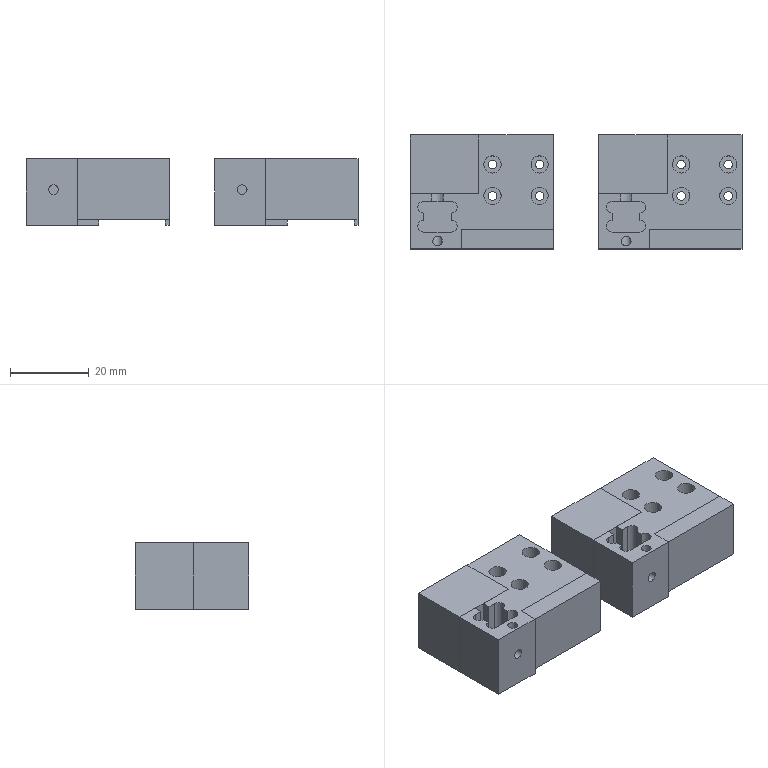NC program | NX | posted with a generic post | part box 84.5 x 29 x 17 mm
Lines 1071 to 2305 of 5162:
(FLOOR_WALL_1 , TOOL : D3)
N2122 T03 M6
N2124 G54
N2126 G17 G0 G90 X-35.75 Y-5.834 B0. C0. S9500 M3
N2128 G43 Z30. H3
N2130 Z1.
N2132 G94 G1 Y-7.2 Z0.928 F1250.
N2134 X-34.75 Z0.876
N2136 Y-5.4 Z0.782
N2138 X-35.75 Z0.729
N2140 Y-7.2 Z0.635
N2142 X-34.75 Z0.583
N2144 Y-5.4 Z0.488
N2146 X-35.75 Z0.436
N2148 Y-7.2 Z0.341
N2150 X-34.75 Z0.289
N2152 Y-5.4 Z0.195
N2154 X-35.75 Z0.142
N2156 Y-7.2 Z0.048
N2158 X-34.75 Z-0.004
N2160 Y-5.4 Z-0.099
N2162 X-35.75 Z-0.151
N2164 Y-6.3 Z-0.198
N2166 Y-7.2
N2168 X-34.75
N2170 Y-5.4
N2172 X-35.75
N2174 Y-6.3
N2176 X-37.25
N2178 Y-7.2
N2180 G2 X-38.75 Y-8.7 R1.5
N2182 G1 X-31.75
N2184 G2 X-33.25 Y-7.2 R1.5
N2186 G1 Y-5.4
N2188 G2 X-31.75 Y-3.9 R1.5
N2190 G1 X-38.75
N2192 G2 X-37.25 Y-5.4 R1.5
N2194 G1 Y-6.3
N2196 Z0.802
N2198 G0 X-35.75 Y-5.834
N2200 G1 Y-7.2 Z0.73
N2202 X-34.75 Z0.678
N2204 Y-5.4 Z0.583
N2206 X-35.75 Z0.531
N2208 Y-7.2 Z0.437
N2210 X-34.75 Z0.384
N2212 Y-5.4 Z0.29
N2214 X-35.75 Z0.237
N2216 Y-7.2 Z0.143
N2218 X-34.75 Z0.091
N2220 Y-5.4 Z-0.004
N2222 X-35.75 Z-0.056
N2224 Y-7.2 Z-0.15
N2226 X-34.75 Z-0.203
N2228 Y-5.4 Z-0.297
N2230 X-35.75 Z-0.35
N2232 Y-6.3 Z-0.397
N2234 Y-7.2
N2236 X-34.75
N2238 Y-5.4
N2240 X-35.75
N2242 Y-6.3
N2244 X-37.25
N2246 Y-7.2
N2248 G2 X-38.75 Y-8.7 R1.5
N2250 G1 X-31.75
N2252 G2 X-33.25 Y-7.2 R1.5
N2254 G1 Y-5.4
N2256 G2 X-31.75 Y-3.9 R1.5
N2258 G1 X-38.75
N2260 G2 X-37.25 Y-5.4 R1.5
N2262 G1 Y-6.3
N2264 Z0.603
N2266 G0 X-35.75 Y-5.834
N2268 G1 Y-7.2 Z0.532
N2270 X-34.75 Z0.479
N2272 Y-5.4 Z0.385
N2274 X-35.75 Z0.333
N2276 Y-7.2 Z0.238
N2278 X-34.75 Z0.186
N2280 Y-5.4 Z0.092
N2282 X-35.75 Z0.039
N2284 Y-7.2 Z-0.055
N2286 X-34.75 Z-0.108
N2288 Y-5.4 Z-0.202
N2290 X-35.75 Z-0.254
N2292 Y-7.2 Z-0.349
N2294 X-34.75 Z-0.401
N2296 Y-5.4 Z-0.495
N2298 X-35.75 Z-0.548
N2300 Y-6.3 Z-0.595
N2302 Y-7.2
N2304 X-34.75
N2306 Y-5.4
N2308 X-35.75
N2310 Y-6.3
N2312 X-37.25
N2314 Y-7.2
N2316 G2 X-38.75 Y-8.7 R1.5
N2318 G1 X-31.75
N2320 G2 X-33.25 Y-7.2 R1.5
N2322 G1 Y-5.4
N2324 G2 X-31.75 Y-3.9 R1.5
N2326 G1 X-38.75
N2328 G2 X-37.25 Y-5.4 R1.5
N2330 G1 Y-6.3
N2332 Z0.405
N2334 G0 X-35.75 Y-5.834
N2336 G1 Y-7.2 Z0.333
N2338 X-34.75 Z0.281
N2340 Y-5.4 Z0.187
N2342 X-35.75 Z0.134
N2344 Y-7.2 Z0.04
N2346 X-34.75 Z-0.012
N2348 Y-5.4 Z-0.107
N2350 X-35.75 Z-0.159
N2352 Y-7.2 Z-0.254
N2354 X-34.75 Z-0.306
N2356 Y-5.4 Z-0.4
N2358 X-35.75 Z-0.453
N2360 Y-7.2 Z-0.547
N2362 X-34.75 Z-0.599
N2364 Y-5.4 Z-0.694
N2366 X-35.75 Z-0.746
N2368 Y-6.3 Z-0.793
N2370 Y-7.2
N2372 X-34.75
N2374 Y-5.4
N2376 X-35.75
N2378 Y-6.3
N2380 X-37.25
N2382 Y-7.2
N2384 G2 X-38.75 Y-8.7 R1.5
N2386 G1 X-31.75
N2388 G2 X-33.25 Y-7.2 R1.5
N2390 G1 Y-5.4
N2392 G2 X-31.75 Y-3.9 R1.5
N2394 G1 X-38.75
N2396 G2 X-37.25 Y-5.4 R1.5
N2398 G1 Y-6.3
N2400 Z0.207
N2402 G0 X-35.75 Y-5.834
N2404 G1 Y-7.2 Z0.135
N2406 X-34.75 Z0.083
N2408 Y-5.4 Z-0.012
N2410 X-35.75 Z-0.064
N2412 Y-7.2 Z-0.158
N2414 X-34.75 Z-0.211
N2416 Y-5.4 Z-0.305
N2418 X-35.75 Z-0.358
N2420 Y-7.2 Z-0.452
N2422 X-34.75 Z-0.504
N2424 Y-5.4 Z-0.599
N2426 X-35.75 Z-0.651
N2428 Y-7.2 Z-0.745
N2430 X-34.75 Z-0.798
N2432 Y-5.4 Z-0.892
N2434 X-35.75 Z-0.945
N2436 Y-6.3 Z-0.992
N2438 Y-7.2
N2440 X-34.75
N2442 Y-5.4
N2444 X-35.75
N2446 Y-6.3
N2448 X-37.25
N2450 Y-7.2
N2452 G2 X-38.75 Y-8.7 R1.5
N2454 G1 X-31.75
N2456 G2 X-33.25 Y-7.2 R1.5
N2458 G1 Y-5.4
N2460 G2 X-31.75 Y-3.9 R1.5
N2462 G1 X-38.75
N2464 G2 X-37.25 Y-5.4 R1.5
N2466 G1 Y-6.3
N2468 Z0.008
N2470 G0 X-35.75 Y-5.834
N2472 G1 Y-7.2 Z-0.063
N2474 X-34.75 Z-0.116
N2476 Y-5.4 Z-0.21
N2478 X-35.75 Z-0.262
N2480 Y-7.2 Z-0.357
N2482 X-34.75 Z-0.409
N2484 Y-5.4 Z-0.503
N2486 X-35.75 Z-0.556
N2488 Y-7.2 Z-0.65
N2490 X-34.75 Z-0.703
N2492 Y-5.4 Z-0.797
N2494 X-35.75 Z-0.849
N2496 Y-7.2 Z-0.944
N2498 X-34.75 Z-0.996
N2500 Y-5.4 Z-1.09
N2502 X-35.75 Z-1.143
N2504 Y-6.3 Z-1.19
N2506 Y-7.2
N2508 X-34.75
N2510 Y-5.4
N2512 X-35.75
N2514 Y-6.3
N2516 X-37.25
N2518 Y-7.2
N2520 G2 X-38.75 Y-8.7 R1.5
N2522 G1 X-31.75
N2524 G2 X-33.25 Y-7.2 R1.5
N2526 G1 Y-5.4
N2528 G2 X-31.75 Y-3.9 R1.5
N2530 G1 X-38.75
N2532 G2 X-37.25 Y-5.4 R1.5
N2534 G1 Y-6.3
N2536 Z-0.19
N2538 G0 X-35.75 Y-5.834
N2540 G1 Y-7.2 Z-0.262
N2542 X-34.75 Z-0.314
N2544 Y-5.4 Z-0.408
N2546 X-35.75 Z-0.461
N2548 Y-7.2 Z-0.555
N2550 X-34.75 Z-0.607
N2552 Y-5.4 Z-0.702
N2554 X-35.75 Z-0.754
N2556 Y-7.2 Z-0.849
N2558 X-34.75 Z-0.901
N2560 Y-5.4 Z-0.995
N2562 X-35.75 Z-1.048
N2564 Y-7.2 Z-1.142
N2566 X-34.75 Z-1.194
N2568 Y-5.4 Z-1.289
N2570 X-35.75 Z-1.341
N2572 Y-6.3 Z-1.388
N2574 Y-7.2
N2576 X-34.75
N2578 Y-5.4
N2580 X-35.75
N2582 Y-6.3
N2584 X-37.25
N2586 Y-7.2
N2588 G2 X-38.75 Y-8.7 R1.5
N2590 G1 X-31.75
N2592 G2 X-33.25 Y-7.2 R1.5
N2594 G1 Y-5.4
N2596 G2 X-31.75 Y-3.9 R1.5
N2598 G1 X-38.75
N2600 G2 X-37.25 Y-5.4 R1.5
N2602 G1 Y-6.3
N2604 Z-0.388
N2606 G0 X-35.75 Y-5.834
N2608 G1 Y-7.2 Z-0.46
N2610 X-34.75 Z-0.512
N2612 Y-5.4 Z-0.607
N2614 X-35.75 Z-0.659
N2616 Y-7.2 Z-0.753
N2618 X-34.75 Z-0.806
N2620 Y-5.4 Z-0.9
N2622 X-35.75 Z-0.953
N2624 Y-7.2 Z-1.047
N2626 X-34.75 Z-1.099
N2628 Y-5.4 Z-1.194
N2630 X-35.75 Z-1.246
N2632 Y-7.2 Z-1.34
N2634 X-34.75 Z-1.393
N2636 Y-5.4 Z-1.487
N2638 X-35.75 Z-1.54
N2640 Y-6.3 Z-1.587
N2642 Y-7.2
N2644 X-34.75
N2646 Y-5.4
N2648 X-35.75
N2650 Y-6.3
N2652 X-37.25
N2654 Y-7.2
N2656 G2 X-38.75 Y-8.7 R1.5
N2658 G1 X-31.75
N2660 G2 X-33.25 Y-7.2 R1.5
N2662 G1 Y-5.4
N2664 G2 X-31.75 Y-3.9 R1.5
N2666 G1 X-38.75
N2668 G2 X-37.25 Y-5.4 R1.5
N2670 G1 Y-6.3
N2672 Z-0.587
N2674 G0 X-35.75 Y-5.834
N2676 G1 Y-7.2 Z-0.658
N2678 X-34.75 Z-0.711
N2680 Y-5.4 Z-0.805
N2682 X-35.75 Z-0.857
N2684 Y-7.2 Z-0.952
N2686 X-34.75 Z-1.004
N2688 Y-5.4 Z-1.098
N2690 X-35.75 Z-1.151
N2692 Y-7.2 Z-1.245
N2694 X-34.75 Z-1.298
N2696 Y-5.4 Z-1.392
N2698 X-35.75 Z-1.444
N2700 Y-7.2 Z-1.539
N2702 X-34.75 Z-1.591
N2704 Y-5.4 Z-1.685
N2706 X-35.75 Z-1.738
N2708 Y-6.3 Z-1.785
N2710 Y-7.2
N2712 X-34.75
N2714 Y-5.4
N2716 X-35.75
N2718 Y-6.3
N2720 X-37.25
N2722 Y-7.2
N2724 G2 X-38.75 Y-8.7 R1.5
N2726 G1 X-31.75
N2728 G2 X-33.25 Y-7.2 R1.5
N2730 G1 Y-5.4
N2732 G2 X-31.75 Y-3.9 R1.5
N2734 G1 X-38.75
N2736 G2 X-37.25 Y-5.4 R1.5
N2738 G1 Y-6.3
N2740 Z-0.785
N2742 G0 X-35.75 Y-5.834
N2744 G1 Y-7.2 Z-0.857
N2746 X-34.75 Z-0.909
N2748 Y-5.4 Z-1.003
N2750 X-35.75 Z-1.056
N2752 Y-7.2 Z-1.15
N2754 X-34.75 Z-1.202
N2756 Y-5.4 Z-1.297
N2758 X-35.75 Z-1.349
N2760 Y-7.2 Z-1.444
N2762 X-34.75 Z-1.496
N2764 Y-5.4 Z-1.59
N2766 X-35.75 Z-1.643
N2768 Y-7.2 Z-1.737
N2770 X-34.75 Z-1.789
N2772 Y-5.4 Z-1.884
N2774 X-35.75 Z-1.936
N2776 Y-6.3 Z-1.983
N2778 Y-7.2
N2780 X-34.75
N2782 Y-5.4
N2784 X-35.75
N2786 Y-6.3
N2788 X-37.25
N2790 Y-7.2
N2792 G2 X-38.75 Y-8.7 R1.5
N2794 G1 X-31.75
N2796 G2 X-33.25 Y-7.2 R1.5
N2798 G1 Y-5.4
N2800 G2 X-31.75 Y-3.9 R1.5
N2802 G1 X-38.75
N2804 G2 X-37.25 Y-5.4 R1.5
N2806 G1 Y-6.3
N2808 Z-0.983
N2810 G0 X-35.75 Y-5.834
N2812 G1 Y-7.2 Z-1.055
N2814 X-34.75 Z-1.107
N2816 Y-5.4 Z-1.202
N2818 X-35.75 Z-1.254
N2820 Y-7.2 Z-1.348
N2822 X-34.75 Z-1.401
N2824 Y-5.4 Z-1.495
N2826 X-35.75 Z-1.548
N2828 Y-7.2 Z-1.642
N2830 X-34.75 Z-1.694
N2832 Y-5.4 Z-1.789
N2834 X-35.75 Z-1.841
N2836 Y-7.2 Z-1.935
N2838 X-34.75 Z-1.988
N2840 Y-5.4 Z-2.082
N2842 X-35.75 Z-2.135
N2844 Y-6.3 Z-2.182
N2846 Y-7.2
N2848 X-34.75
N2850 Y-5.4
N2852 X-35.75
N2854 Y-6.3
N2856 X-37.25
N2858 Y-7.2
N2860 G2 X-38.75 Y-8.7 R1.5
N2862 G1 X-31.75
N2864 G2 X-33.25 Y-7.2 R1.5
N2866 G1 Y-5.4
N2868 G2 X-31.75 Y-3.9 R1.5
N2870 G1 X-38.75
N2872 G2 X-37.25 Y-5.4 R1.5
N2874 G1 Y-6.3
N2876 Z-1.182
N2878 G0 X-35.75 Y-5.834
N2880 G1 Y-7.2 Z-1.253
N2882 X-34.75 Z-1.306
N2884 Y-5.4 Z-1.4
N2886 X-35.75 Z-1.452
N2888 Y-7.2 Z-1.547
N2890 X-34.75 Z-1.599
N2892 Y-5.4 Z-1.693
N2894 X-35.75 Z-1.746
N2896 Y-7.2 Z-1.84
N2898 X-34.75 Z-1.893
N2900 Y-5.4 Z-1.987
N2902 X-35.75 Z-2.039
N2904 Y-7.2 Z-2.134
N2906 X-34.75 Z-2.186
N2908 Y-5.4 Z-2.28
N2910 X-35.75 Z-2.333
N2912 Y-6.3 Z-2.38
N2914 Y-7.2
N2916 X-34.75
N2918 Y-5.4
N2920 X-35.75
N2922 Y-6.3
N2924 X-37.25
N2926 Y-7.2
N2928 G2 X-38.75 Y-8.7 R1.5
N2930 G1 X-31.75
N2932 G2 X-33.25 Y-7.2 R1.5
N2934 G1 Y-5.4
N2936 G2 X-31.75 Y-3.9 R1.5
N2938 G1 X-38.75
N2940 G2 X-37.25 Y-5.4 R1.5
N2942 G1 Y-6.3
N2944 Z-1.38
N2946 G0 X-35.75 Y-5.834
N2948 G1 Y-7.2 Z-1.452
N2950 X-34.75 Z-1.504
N2952 Y-5.4 Z-1.598
N2954 X-35.75 Z-1.651
N2956 Y-7.2 Z-1.745
N2958 X-34.75 Z-1.797
N2960 Y-5.4 Z-1.892
N2962 X-35.75 Z-1.944
N2964 Y-7.2 Z-2.039
N2966 X-34.75 Z-2.091
N2968 Y-5.4 Z-2.185
N2970 X-35.75 Z-2.238
N2972 Y-7.2 Z-2.332
N2974 X-34.75 Z-2.384
N2976 Y-5.4 Z-2.479
N2978 X-35.75 Z-2.531
N2980 Y-6.3 Z-2.578
N2982 Y-7.2
N2984 X-34.75
N2986 Y-5.4
N2988 X-35.75
N2990 Y-6.3
N2992 X-37.25
N2994 Y-7.2
N2996 G2 X-38.75 Y-8.7 R1.5
N2998 G1 X-31.75
N3000 G2 X-33.25 Y-7.2 R1.5
N3002 G1 Y-5.4
N3004 G2 X-31.75 Y-3.9 R1.5
N3006 G1 X-38.75
N3008 G2 X-37.25 Y-5.4 R1.5
N3010 G1 Y-6.3
N3012 Z-1.578
N3014 G0 X-35.75 Y-5.834
N3016 G1 Y-7.2 Z-1.65
N3018 X-34.75 Z-1.702
N3020 Y-5.4 Z-1.797
N3022 X-35.75 Z-1.849
N3024 Y-7.2 Z-1.943
N3026 X-34.75 Z-1.996
N3028 Y-5.4 Z-2.09
N3030 X-35.75 Z-2.143
N3032 Y-7.2 Z-2.237
N3034 X-34.75 Z-2.289
N3036 Y-5.4 Z-2.384
N3038 X-35.75 Z-2.436
N3040 Y-7.2 Z-2.53
N3042 X-34.75 Z-2.583
N3044 Y-5.4 Z-2.677
N3046 X-35.75 Z-2.73
N3048 Y-6.3 Z-2.777
N3050 Y-7.2
N3052 X-34.75
N3054 Y-5.4
N3056 X-35.75
N3058 Y-6.3
N3060 X-37.25
N3062 Y-7.2
N3064 G2 X-38.75 Y-8.7 R1.5
N3066 G1 X-31.75
N3068 G2 X-33.25 Y-7.2 R1.5
N3070 G1 Y-5.4
N3072 G2 X-31.75 Y-3.9 R1.5
N3074 G1 X-38.75
N3076 G2 X-37.25 Y-5.4 R1.5
N3078 G1 Y-6.3
N3080 Z-1.777
N3082 G0 X-35.75 Y-5.834
N3084 G1 Y-7.2 Z-1.848
N3086 X-34.75 Z-1.901
N3088 Y-5.4 Z-1.995
N3090 X-35.75 Z-2.047
N3092 Y-7.2 Z-2.142
N3094 X-34.75 Z-2.194
N3096 Y-5.4 Z-2.288
N3098 X-35.75 Z-2.341
N3100 Y-7.2 Z-2.435
N3102 X-34.75 Z-2.488
N3104 Y-5.4 Z-2.582
N3106 X-35.75 Z-2.634
N3108 Y-7.2 Z-2.729
N3110 X-34.75 Z-2.781
N3112 Y-5.4 Z-2.875
N3114 X-35.75 Z-2.928
N3116 Y-6.3 Z-2.975
N3118 Y-7.2
N3120 X-34.75
N3122 Y-5.4
N3124 X-35.75
N3126 Y-6.3
N3128 X-37.25
N3130 Y-7.2
N3132 G2 X-38.75 Y-8.7 R1.5
N3134 G1 X-31.75
N3136 G2 X-33.25 Y-7.2 R1.5
N3138 G1 Y-5.4
N3140 G2 X-31.75 Y-3.9 R1.5
N3142 G1 X-38.75
N3144 G2 X-37.25 Y-5.4 R1.5
N3146 G1 Y-6.3
N3148 Z-1.975
N3150 G0 X-35.75 Y-5.834
N3152 G1 Y-7.2 Z-2.047
N3154 X-34.75 Z-2.099
N3156 Y-5.4 Z-2.193
N3158 X-35.75 Z-2.246
N3160 Y-7.2 Z-2.34
N3162 X-34.75 Z-2.392
N3164 Y-5.4 Z-2.487
N3166 X-35.75 Z-2.539
N3168 Y-7.2 Z-2.634
N3170 X-34.75 Z-2.686
N3172 Y-5.4 Z-2.78
N3174 X-35.75 Z-2.833
N3176 Y-7.2 Z-2.927
N3178 X-34.75 Z-2.979
N3180 Y-5.4 Z-3.074
N3182 X-35.75 Z-3.126
N3184 Y-6.3 Z-3.173
N3186 Y-7.2
N3188 X-34.75
N3190 Y-5.4
N3192 X-35.75
N3194 Y-6.3
N3196 X-37.25
N3198 Y-7.2
N3200 G2 X-38.75 Y-8.7 R1.5
N3202 G1 X-31.75
N3204 G2 X-33.25 Y-7.2 R1.5
N3206 G1 Y-5.4
N3208 G2 X-31.75 Y-3.9 R1.5
N3210 G1 X-38.75
N3212 G2 X-37.25 Y-5.4 R1.5
N3214 G1 Y-6.3
N3216 Z-2.173
N3218 G0 X-35.75 Y-5.834
N3220 G1 Y-7.2 Z-2.245
N3222 X-34.75 Z-2.297
N3224 Y-5.4 Z-2.392
N3226 X-35.75 Z-2.444
N3228 Y-7.2 Z-2.538
N3230 X-34.75 Z-2.591
N3232 Y-5.4 Z-2.685
N3234 X-35.75 Z-2.738
N3236 Y-7.2 Z-2.832
N3238 X-34.75 Z-2.884
N3240 Y-5.4 Z-2.979
N3242 X-35.75 Z-3.031
N3244 Y-7.2 Z-3.125
N3246 X-34.75 Z-3.178
N3248 Y-5.4 Z-3.272
N3250 X-35.75 Z-3.325
N3252 Y-6.3 Z-3.372
N3254 Y-7.2
N3256 X-34.75
N3258 Y-5.4
N3260 X-35.75
N3262 Y-6.3
N3264 X-37.25
N3266 Y-7.2
N3268 G2 X-38.75 Y-8.7 R1.5
N3270 G1 X-31.75
N3272 G2 X-33.25 Y-7.2 R1.5
N3274 G1 Y-5.4
N3276 G2 X-31.75 Y-3.9 R1.5
N3278 G1 X-38.75
N3280 G2 X-37.25 Y-5.4 R1.5
N3282 G1 Y-6.3
N3284 Z-2.372
N3286 G0 X-35.75 Y-5.834
N3288 G1 Y-7.2 Z-2.443
N3290 X-34.75 Z-2.496
N3292 Y-5.4 Z-2.59
N3294 X-35.75 Z-2.642
N3296 Y-7.2 Z-2.737
N3298 X-34.75 Z-2.789
N3300 Y-5.4 Z-2.883
N3302 X-35.75 Z-2.936
N3304 Y-7.2 Z-3.03
N3306 X-34.75 Z-3.083
N3308 Y-5.4 Z-3.177
N3310 X-35.75 Z-3.229
N3312 Y-7.2 Z-3.324
N3314 X-34.75 Z-3.376
N3316 Y-5.4 Z-3.47
N3318 X-35.75 Z-3.523
N3320 Y-6.3 Z-3.57
N3322 Y-7.2
N3324 X-34.75
N3326 Y-5.4
N3328 X-35.75
N3330 Y-6.3
N3332 X-37.25
N3334 Y-7.2
N3336 G2 X-38.75 Y-8.7 R1.5
N3338 G1 X-31.75
N3340 G2 X-33.25 Y-7.2 R1.5
N3342 G1 Y-5.4
N3344 G2 X-31.75 Y-3.9 R1.5
N3346 G1 X-38.75
N3348 G2 X-37.25 Y-5.4 R1.5
N3350 G1 Y-6.3
N3352 Z-2.57
N3354 G0 X-35.75 Y-5.834
N3356 G1 Y-7.2 Z-2.642
N3358 X-34.75 Z-2.694
N3360 Y-5.4 Z-2.788
N3362 X-35.75 Z-2.841
N3364 Y-7.2 Z-2.935
N3366 X-34.75 Z-2.987
N3368 Y-5.4 Z-3.082
N3370 X-35.75 Z-3.134
N3372 Y-7.2 Z-3.229
N3374 X-34.75 Z-3.281
N3376 Y-5.4 Z-3.375
N3378 X-35.75 Z-3.428
N3380 Y-7.2 Z-3.522
N3382 X-34.75 Z-3.574
N3384 Y-5.4 Z-3.669
N3386 X-35.75 Z-3.721
N3388 Y-6.3 Z-3.768
N3390 Y-7.2
N3392 X-34.75
N3394 Y-5.4
N3396 X-35.75
N3398 Y-6.3
N3400 X-37.25
N3402 Y-7.2
N3404 G2 X-38.75 Y-8.7 R1.5
N3406 G1 X-31.75
N3408 G2 X-33.25 Y-7.2 R1.5
N3410 G1 Y-5.4
N3412 G2 X-31.75 Y-3.9 R1.5
N3414 G1 X-38.75
N3416 G2 X-37.25 Y-5.4 R1.5
N3418 G1 Y-6.3
N3420 Z-2.768
N3422 G0 X-35.75 Y-5.834
N3424 G1 Y-7.2 Z-2.84
N3426 X-34.75 Z-2.892
N3428 Y-5.4 Z-2.987
N3430 X-35.75 Z-3.039
N3432 Y-7.2 Z-3.133
N3434 X-34.75 Z-3.186
N3436 Y-5.4 Z-3.28
N3438 X-35.75 Z-3.333
N3440 Y-7.2 Z-3.427
N3442 X-34.75 Z-3.479
N3444 Y-5.4 Z-3.574
N3446 X-35.75 Z-3.626
N3448 Y-7.2 Z-3.72
N3450 X-34.75 Z-3.773
N3452 Y-5.4 Z-3.867
N3454 X-35.75 Z-3.92
N3456 Y-6.3 Z-3.967
N3458 Y-7.2
N3460 X-34.75
N3462 Y-5.4
N3464 X-35.75
N3466 Y-6.3
N3468 X-37.25
N3470 Y-7.2
N3472 G2 X-38.75 Y-8.7 R1.5
N3474 G1 X-31.75
N3476 G2 X-33.25 Y-7.2 R1.5
N3478 G1 Y-5.4
N3480 G2 X-31.75 Y-3.9 R1.5
N3482 G1 X-38.75
N3484 G2 X-37.25 Y-5.4 R1.5
N3486 G1 Y-6.3
N3488 Z-2.967
N3490 G0 X-35.75 Y-5.834
N3492 G1 Y-7.2 Z-3.038
N3494 X-34.75 Z-3.091
N3496 Y-5.4 Z-3.185
N3498 X-35.75 Z-3.237
N3500 Y-7.2 Z-3.332
N3502 X-34.75 Z-3.384
N3504 Y-5.4 Z-3.478
N3506 X-35.75 Z-3.531
N3508 Y-7.2 Z-3.625
N3510 X-34.75 Z-3.678
N3512 Y-5.4 Z-3.772
N3514 X-35.75 Z-3.824
N3516 Y-7.2 Z-3.919
N3518 X-34.75 Z-3.971
N3520 Y-5.4 Z-4.065
N3522 X-35.75 Z-4.118
N3524 Y-6.3 Z-4.165
N3526 Y-7.2
N3528 X-34.75
N3530 Y-5.4
N3532 X-35.75
N3534 Y-6.3
N3536 X-37.25
N3538 Y-7.2
N3540 G2 X-38.75 Y-8.7 R1.5
N3542 G1 X-31.75
N3544 G2 X-33.25 Y-7.2 R1.5
N3546 G1 Y-5.4
N3548 G2 X-31.75 Y-3.9 R1.5
N3550 G1 X-38.75
N3552 G2 X-37.25 Y-5.4 R1.5
N3554 G1 Y-6.3
N3556 Z-3.165
N3558 G0 X-35.75 Y-5.834
N3560 G1 Y-7.2 Z-3.237
N3562 X-34.75 Z-3.289
N3564 Y-5.4 Z-3.383
N3566 X-35.75 Z-3.436
N3568 Y-7.2 Z-3.53
N3570 X-34.75 Z-3.582
N3572 Y-5.4 Z-3.677
N3574 X-35.75 Z-3.729
N3576 Y-7.2 Z-3.824
N3578 X-34.75 Z-3.876
N3580 Y-5.4 Z-3.97
N3582 X-35.75 Z-4.023
N3584 Y-7.2 Z-4.117
N3586 X-34.75 Z-4.169
N3588 Y-5.4 Z-4.264
N3590 X-35.75 Z-4.316
N3592 Y-6.3 Z-4.363
N3594 Y-7.2
N3596 X-34.75
N3598 Y-5.4
N3600 X-35.75
N3602 Y-6.3
N3604 X-37.25
N3606 Y-7.2
N3608 G2 X-38.75 Y-8.7 R1.5
N3610 G1 X-31.75
N3612 G2 X-33.25 Y-7.2 R1.5
N3614 G1 Y-5.4
N3616 G2 X-31.75 Y-3.9 R1.5
N3618 G1 X-38.75
N3620 G2 X-37.25 Y-5.4 R1.5
N3622 G1 Y-6.3
N3624 Z-3.363
N3626 G0 X-35.75 Y-5.834
N3628 G1 Y-7.2 Z-3.435
N3630 X-34.75 Z-3.487
N3632 Y-5.4 Z-3.582
N3634 X-35.75 Z-3.634
N3636 Y-7.2 Z-3.728
N3638 X-34.75 Z-3.781
N3640 Y-5.4 Z-3.875
N3642 X-35.75 Z-3.928
N3644 Y-7.2 Z-4.022
N3646 X-34.75 Z-4.074
N3648 Y-5.4 Z-4.169
N3650 X-35.75 Z-4.221
N3652 Y-7.2 Z-4.315
N3654 X-34.75 Z-4.368
N3656 Y-5.4 Z-4.462
N3658 X-35.75 Z-4.515
N3660 Y-6.3 Z-4.562
N3662 Y-7.2
N3664 X-34.75
N3666 Y-5.4
N3668 X-35.75
N3670 Y-6.3
N3672 X-37.25
N3674 Y-7.2
N3676 G2 X-38.75 Y-8.7 R1.5
N3678 G1 X-31.75
N3680 G2 X-33.25 Y-7.2 R1.5
N3682 G1 Y-5.4
N3684 G2 X-31.75 Y-3.9 R1.5
N3686 G1 X-38.75
N3688 G2 X-37.25 Y-5.4 R1.5
N3690 G1 Y-6.3
N3692 Z-3.562
N3694 G0 X-35.75 Y-5.834
N3696 G1 Y-7.2 Z-3.633
N3698 X-34.75 Z-3.686
N3700 Y-5.4 Z-3.78
N3702 X-35.75 Z-3.832
N3704 Y-7.2 Z-3.927
N3706 X-34.75 Z-3.979
N3708 Y-5.4 Z-4.073
N3710 X-35.75 Z-4.126
N3712 Y-7.2 Z-4.22
N3714 X-34.75 Z-4.273
N3716 Y-5.4 Z-4.367
N3718 X-35.75 Z-4.419
N3720 Y-7.2 Z-4.514
N3722 X-34.75 Z-4.566
N3724 Y-5.4 Z-4.66
N3726 X-35.75 Z-4.713
N3728 Y-6.3 Z-4.76
N3730 Y-7.2
N3732 X-34.75
N3734 Y-5.4
N3736 X-35.75
N3738 Y-6.3
N3740 X-37.25
N3742 Y-7.2
N3744 G2 X-38.75 Y-8.7 R1.5
N3746 G1 X-31.75
N3748 G2 X-33.25 Y-7.2 R1.5
N3750 G1 Y-5.4
N3752 G2 X-31.75 Y-3.9 R1.5
N3754 G1 X-38.75
N3756 G2 X-37.25 Y-5.4 R1.5
N3758 G1 Y-6.3
N3760 Z-3.76
N3762 G0 X-35.75 Y-5.834
N3764 G1 Y-7.2 Z-3.832
N3766 X-34.75 Z-3.884
N3768 Y-5.4 Z-3.978
N3770 X-35.75 Z-4.031
N3772 Y-7.2 Z-4.125
N3774 X-34.75 Z-4.177
N3776 Y-5.4 Z-4.272
N3778 X-35.75 Z-4.324
N3780 Y-7.2 Z-4.419
N3782 X-34.75 Z-4.471
N3784 Y-5.4 Z-4.565
N3786 X-35.75 Z-4.618
N3788 Y-7.2 Z-4.712
N3790 X-34.75 Z-4.764
N3792 Y-5.4 Z-4.859
N3794 X-35.75 Z-4.911
N3796 Y-6.3 Z-4.958
N3798 Y-7.2
N3800 X-34.75
N3802 Y-5.4
N3804 X-35.75
N3806 Y-6.3
N3808 X-37.25
N3810 Y-7.2
N3812 G2 X-38.75 Y-8.7 R1.5
N3814 G1 X-31.75
N3816 G2 X-33.25 Y-7.2 R1.5
N3818 G1 Y-5.4
N3820 G2 X-31.75 Y-3.9 R1.5
N3822 G1 X-38.75
N3824 G2 X-37.25 Y-5.4 R1.5
N3826 G1 Y-6.3
N3828 Z-3.958
N3830 G0 X-35.75 Y-5.834
N3832 G1 Y-7.2 Z-4.03
N3834 X-34.75 Z-4.082
N3836 Y-5.4 Z-4.177
N3838 X-35.75 Z-4.229
N3840 Y-7.2 Z-4.323
N3842 X-34.75 Z-4.376
N3844 Y-5.4 Z-4.47
N3846 X-35.75 Z-4.523
N3848 Y-7.2 Z-4.617
N3850 X-34.75 Z-4.669
N3852 Y-5.4 Z-4.764
N3854 X-35.75 Z-4.816
N3856 Y-7.2 Z-4.91
N3858 X-34.75 Z-4.963
N3860 Y-5.4 Z-5.057
N3862 X-35.75 Z-5.11
N3864 Y-6.3 Z-5.157
N3866 Y-7.2
N3868 X-34.75
N3870 Y-5.4
N3872 X-35.75
N3874 Y-6.3
N3876 X-37.25
N3878 Y-7.2
N3880 G2 X-38.75 Y-8.7 R1.5
N3882 G1 X-31.75
N3884 G2 X-33.25 Y-7.2 R1.5
N3886 G1 Y-5.4
N3888 G2 X-31.75 Y-3.9 R1.5
N3890 G1 X-38.75
N3892 G2 X-37.25 Y-5.4 R1.5
N3894 G1 Y-6.3
N3896 Z-4.157
N3898 G0 X-35.75 Y-5.834
N3900 G1 Y-7.2 Z-4.228
N3902 X-34.75 Z-4.281
N3904 Y-5.4 Z-4.375
N3906 X-35.75 Z-4.427
N3908 Y-7.2 Z-4.522
N3910 X-34.75 Z-4.574
N3912 Y-5.4 Z-4.668
N3914 X-35.75 Z-4.721
N3916 Y-7.2 Z-4.815
N3918 X-34.75 Z-4.868
N3920 Y-5.4 Z-4.962
N3922 X-35.75 Z-5.014
N3924 Y-7.2 Z-5.109
N3926 X-34.75 Z-5.161
N3928 Y-5.4 Z-5.255
N3930 X-35.75 Z-5.308
N3932 Y-6.3 Z-5.355
N3934 Y-7.2
N3936 X-34.75
N3938 Y-5.4
N3940 X-35.75
N3942 Y-6.3
N3944 X-37.25
N3946 Y-7.2
N3948 G2 X-38.75 Y-8.7 R1.5
N3950 G1 X-31.75
N3952 G2 X-33.25 Y-7.2 R1.5
N3954 G1 Y-5.4
N3956 G2 X-31.75 Y-3.9 R1.5
N3958 G1 X-38.75
N3960 G2 X-37.25 Y-5.4 R1.5
N3962 G1 Y-6.3
N3964 Z-4.355
N3966 G0 X-35.75 Y-5.834
N3968 G1 Y-7.2 Z-4.427
N3970 X-34.75 Z-4.479
N3972 Y-5.4 Z-4.573
N3974 X-35.75 Z-4.626
N3976 Y-7.2 Z-4.72
N3978 X-34.75 Z-4.772
N3980 Y-5.4 Z-4.867
N3982 X-35.75 Z-4.919
N3984 Y-7.2 Z-5.014
N3986 X-34.75 Z-5.066
N3988 Y-5.4 Z-5.16
N3990 X-35.75 Z-5.213
N3992 Y-7.2 Z-5.307
N3994 X-34.75 Z-5.359
N3996 Y-5.4 Z-5.454
N3998 X-35.75 Z-5.506
N4000 Y-6.3 Z-5.553
N4002 Y-7.2
N4004 X-34.75
N4006 Y-5.4
N4008 X-35.75
N4010 Y-6.3
N4012 X-37.25
N4014 Y-7.2
N4016 G2 X-38.75 Y-8.7 R1.5
N4018 G1 X-31.75
N4020 G2 X-33.25 Y-7.2 R1.5
N4022 G1 Y-5.4
N4024 G2 X-31.75 Y-3.9 R1.5
N4026 G1 X-38.75
N4028 G2 X-37.25 Y-5.4 R1.5
N4030 G1 Y-6.3
N4032 Z-4.553
N4034 G0 X-35.75 Y-5.834
N4036 G1 Y-7.2 Z-4.625
N4038 X-34.75 Z-4.677
N4040 Y-5.4 Z-4.772
N4042 X-35.75 Z-4.824
N4044 Y-7.2 Z-4.918
N4046 X-34.75 Z-4.971
N4048 Y-5.4 Z-5.065
N4050 X-35.75 Z-5.118
N4052 Y-7.2 Z-5.212
N4054 X-34.75 Z-5.264
N4056 Y-5.4 Z-5.359
N4058 X-35.75 Z-5.411
N4060 Y-7.2 Z-5.505
N4062 X-34.75 Z-5.558
N4064 Y-5.4 Z-5.652
N4066 X-35.75 Z-5.705
N4068 Y-6.3 Z-5.752
N4070 Y-7.2
N4072 X-34.75
N4074 Y-5.4
N4076 X-35.75
N4078 Y-6.3
N4080 X-37.25
N4082 Y-7.2
N4084 G2 X-38.75 Y-8.7 R1.5
N4086 G1 X-31.75
N4088 G2 X-33.25 Y-7.2 R1.5
N4090 G1 Y-5.4
N4092 G2 X-31.75 Y-3.9 R1.5
N4094 G1 X-38.75
N4096 G2 X-37.25 Y-5.4 R1.5
N4098 G1 Y-6.3
N4100 Z-4.752
N4102 G0 X-35.75 Y-5.834
N4104 G1 Y-7.2 Z-4.823
N4106 X-34.75 Z-4.876
N4108 Y-5.4 Z-4.97
N4110 X-35.75 Z-5.022
N4112 Y-7.2 Z-5.117
N4114 X-34.75 Z-5.169
N4116 Y-5.4 Z-5.263
N4118 X-35.75 Z-5.316
N4120 Y-7.2 Z-5.41
N4122 X-34.75 Z-5.463
N4124 Y-5.4 Z-5.557
N4126 X-35.75 Z-5.609
N4128 Y-7.2 Z-5.704
N4130 X-34.75 Z-5.756
N4132 Y-5.4 Z-5.85
N4134 X-35.75 Z-5.903
N4136 Y-6.3 Z-5.95
N4138 Y-7.2
N4140 X-34.75
N4142 Y-5.4
N4144 X-35.75
N4146 Y-6.3
N4148 X-37.25
N4150 Y-7.2
N4152 G2 X-38.75 Y-8.7 R1.5
N4154 G1 X-31.75
N4156 G2 X-33.25 Y-7.2 R1.5
N4158 G1 Y-5.4
N4160 G2 X-31.75 Y-3.9 R1.5
N4162 G1 X-38.75
N4164 G2 X-37.25 Y-5.4 R1.5
N4166 G1 Y-6.3
N4168 Z-4.95
N4170 G0 X-35.75 Y-5.834
N4172 G1 Y-7.2 Z-5.022
N4174 X-34.75 Z-5.074
N4176 Y-5.4 Z-5.168
N4178 X-35.75 Z-5.221
N4180 Y-7.2 Z-5.315
N4182 X-34.75 Z-5.367
N4184 Y-5.4 Z-5.462
N4186 X-35.75 Z-5.514
N4188 Y-7.2 Z-5.609
N4190 X-34.75 Z-5.661
N4192 Y-5.4 Z-5.755
N4194 X-35.75 Z-5.808
N4196 Y-7.2 Z-5.902
N4198 X-34.75 Z-5.954
N4200 Y-5.4 Z-6.049
N4202 X-35.75 Z-6.101
N4204 Y-6.3 Z-6.148
N4206 Y-7.2
N4208 X-34.75
N4210 Y-5.4
N4212 X-35.75
N4214 Y-6.3
N4216 X-37.25
N4218 Y-7.2
N4220 G2 X-38.75 Y-8.7 R1.5
N4222 G1 X-31.75
N4224 G2 X-33.25 Y-7.2 R1.5
N4226 G1 Y-5.4
N4228 G2 X-31.75 Y-3.9 R1.5
N4230 G1 X-38.75
N4232 G2 X-37.25 Y-5.4 R1.5
N4234 G1 Y-6.3
N4236 Z-5.148
N4238 G0 X-35.75 Y-5.834
N4240 G1 Y-7.2 Z-5.22
N4242 X-34.75 Z-5.272
N4244 Y-5.4 Z-5.367
N4246 X-35.75 Z-5.419
N4248 Y-7.2 Z-5.513
N4250 X-34.75 Z-5.566
N4252 Y-5.4 Z-5.66
N4254 X-35.75 Z-5.713
N4256 Y-7.2 Z-5.807
N4258 X-34.75 Z-5.859
N4260 Y-5.4 Z-5.954
N4262 X-35.75 Z-6.006
N4264 Y-7.2 Z-6.1
N4266 X-34.75 Z-6.153
N4268 Y-5.4 Z-6.247
N4270 X-35.75 Z-6.3
N4272 Y-6.3 Z-6.347
N4274 Y-7.2
N4276 X-34.75
N4278 Y-5.4
N4280 X-35.75
N4282 Y-6.3
N4284 X-37.25
N4286 Y-7.2
N4288 G2 X-38.75 Y-8.7 R1.5
N4290 G1 X-31.75
N4292 G2 X-33.25 Y-7.2 R1.5
N4294 G1 Y-5.4
N4296 G2 X-31.75 Y-3.9 R1.5
N4298 G1 X-38.75
N4300 G2 X-37.25 Y-5.4 R1.5
N4302 G1 Y-6.3
N4304 Z-5.347
N4306 G0 X-35.75 Y-5.834
N4308 G1 Y-7.2 Z-5.418
N4310 X-34.75 Z-5.471
N4312 Y-5.4 Z-5.565
N4314 X-35.75 Z-5.617
N4316 Y-7.2 Z-5.712
N4318 X-34.75 Z-5.764
N4320 Y-5.4 Z-5.858
N4322 X-35.75 Z-5.911
N4324 Y-7.2 Z-6.005
N4326 X-34.75 Z-6.058
N4328 Y-5.4 Z-6.152
N4330 X-35.75 Z-6.204
N4332 Y-7.2 Z-6.299
N4334 X-34.75 Z-6.351
N4336 Y-5.4 Z-6.445
N4338 X-35.75 Z-6.498
N4340 Y-6.3 Z-6.545
N4342 Y-7.2
N4344 X-34.75
N4346 Y-5.4
N4348 X-35.75
N4350 Y-6.3
N4352 X-37.25
N4354 Y-7.2
N4356 G2 X-38.75 Y-8.7 R1.5
N4358 G1 X-31.75
N4360 G2 X-33.25 Y-7.2 R1.5
N4362 G1 Y-5.4
N4364 G2 X-31.75 Y-3.9 R1.5
N4366 G1 X-38.75
N4368 G2 X-37.25 Y-5.4 R1.5
N4370 G1 Y-6.3
N4372 Z-5.545
N4374 G0 X-35.75 Y-5.834
N4376 G1 Y-7.2 Z-5.617
N4378 X-34.75 Z-5.669
N4380 Y-5.4 Z-5.763
N4382 X-35.75 Z-5.816
N4384 Y-7.2 Z-5.91
N4386 X-34.75 Z-5.962
N4388 Y-5.4 Z-6.057
N4390 X-35.75 Z-6.109
N4392 Y-7.2 Z-6.204
N4394 X-34.75 Z-6.256
N4396 Y-5.4 Z-6.35
N4398 X-35.75 Z-6.403
N4400 Y-7.2 Z-6.497
N4402 X-34.75 Z-6.549
N4404 Y-5.4 Z-6.644
N4406 X-35.75 Z-6.696
N4408 Y-6.3 Z-6.743
N4410 Y-7.2
N4412 X-34.75
N4414 Y-5.4
N4416 X-35.75
N4418 Y-6.3
N4420 X-37.25
N4422 Y-7.2
N4424 G2 X-38.75 Y-8.7 R1.5
N4426 G1 X-31.75
N4428 G2 X-33.25 Y-7.2 R1.5
N4430 G1 Y-5.4
N4432 G2 X-31.75 Y-3.9 R1.5
N4434 G1 X-38.75
N4436 G2 X-37.25 Y-5.4 R1.5
N4438 G1 Y-6.3
N4440 Z-5.743
N4442 G0 X-35.75 Y-5.834
N4444 G1 Y-7.2 Z-5.815
N4446 X-34.75 Z-5.867
N4448 Y-5.4 Z-5.962
N4450 X-35.75 Z-6.014
N4452 Y-7.2 Z-6.108
N4454 X-34.75 Z-6.161
N4456 Y-5.4 Z-6.255
N4458 X-35.75 Z-6.308
N4460 Y-7.2 Z-6.402
N4462 X-34.75 Z-6.454
N4464 Y-5.4 Z-6.549
N4466 X-35.75 Z-6.601
N4468 Y-7.2 Z-6.695
N4470 X-34.75 Z-6.748
N4472 Y-5.4 Z-6.842
N4474 X-35.75 Z-6.895
N4476 Y-6.3 Z-6.942
N4478 Y-7.2
N4480 X-34.75
N4482 Y-5.4
N4484 X-35.75
N4486 Y-6.3
N4488 X-37.25
N4490 Y-7.2
N4492 G2 X-38.75 Y-8.7 R1.5
N4494 G1 X-31.75
N4496 G2 X-33.25 Y-7.2 R1.5
N4498 G1 Y-5.4
N4500 G2 X-31.75 Y-3.9 R1.5
N4502 G1 X-38.75
N4504 G2 X-37.25 Y-5.4 R1.5
N4506 G1 Y-6.3
N4508 Z-5.942
N4510 G0 X-35.75 Y-5.834
N4512 G1 Y-7.2 Z-6.013
N4514 X-34.75 Z-6.066
N4516 Y-5.4 Z-6.16
N4518 X-35.75 Z-6.212
N4520 Y-7.2 Z-6.307
N4522 X-34.75 Z-6.359
N4524 Y-5.4 Z-6.453
N4526 X-35.75 Z-6.506
N4528 Y-7.2 Z-6.6
N4530 X-34.75 Z-6.653
N4532 Y-5.4 Z-6.747
N4534 X-35.75 Z-6.799
N4536 Y-7.2 Z-6.894
N4538 X-34.75 Z-6.946
N4540 Y-5.4 Z-7.04
N4542 X-35.75 Z-7.093
N4544 Y-6.3 Z-7.14
N4546 Y-7.2
N4548 X-34.75
N4550 Y-5.4
N4552 X-35.75
N4554 Y-6.3
N4556 X-37.25
N4558 Y-7.2
N4560 G2 X-38.75 Y-8.7 R1.5
N4562 G1 X-31.75
N4564 G2 X-33.25 Y-7.2 R1.5
N4566 G1 Y-5.4
N4568 G2 X-31.75 Y-3.9 R1.5
N4570 G1 X-38.75
N4572 G2 X-37.25 Y-5.4 R1.5
N4574 G1 Y-6.3
N4576 Z-6.14
N4578 G0 X-35.75 Y-5.834
N4580 G1 Y-7.2 Z-6.212
N4582 X-34.75 Z-6.264
N4584 Y-5.4 Z-6.358